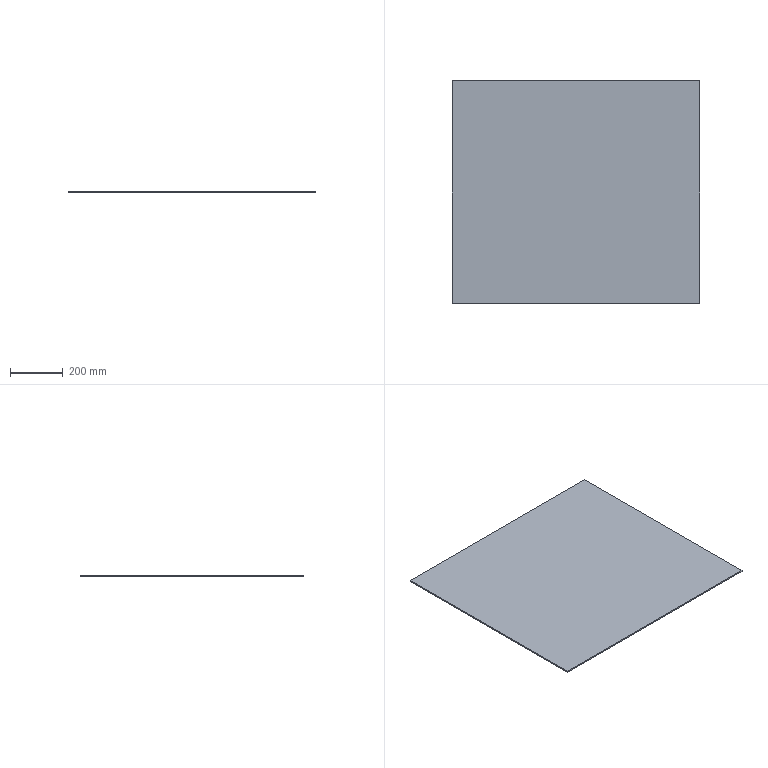Part | SolidWorks | features Extrusion 1, HoleWzd 1 | 1 solid | 6 faces | box 936 x 842 x 5 mm | volume 3940560 mm3 | plane 6
STEP:
#1=CARTESIAN_POINT('',(468.,-421.,0.));
#2=VERTEX_POINT('',#1);
#3=CARTESIAN_POINT('',(468.,421.,0.));
#4=VERTEX_POINT('',#3);
#5=CARTESIAN_POINT('',(468.,421.,0.));
#6=DIRECTION('',(0.,1.,0.));
#7=VECTOR('',#6,1000.);
#8=LINE('',#5,#7);
#9=EDGE_CURVE('',#2,#4,#8,.T.);
#10=ORIENTED_EDGE('',*,*,#9,.T.);
#11=CARTESIAN_POINT('',(468.,421.,5.));
#12=VERTEX_POINT('',#11);
#13=CARTESIAN_POINT('',(468.,421.,5.));
#14=DIRECTION('',(0.,0.,-1.));
#15=VECTOR('',#14,1000.);
#16=LINE('',#13,#15);
#17=EDGE_CURVE('',#12,#4,#16,.T.);
#18=ORIENTED_EDGE('',*,*,#17,.F.);
#19=CARTESIAN_POINT('',(468.,-421.,5.));
#20=VERTEX_POINT('',#19);
#21=CARTESIAN_POINT('',(468.,421.,5.));
#22=DIRECTION('',(0.,1.,0.));
#23=VECTOR('',#22,1000.);
#24=LINE('',#21,#23);
#25=EDGE_CURVE('',#20,#12,#24,.T.);
#26=ORIENTED_EDGE('',*,*,#25,.F.);
#27=CARTESIAN_POINT('',(468.,-421.,5.));
#28=DIRECTION('',(0.,0.,-1.));
#29=VECTOR('',#28,1000.);
#30=LINE('',#27,#29);
#31=EDGE_CURVE('',#20,#2,#30,.T.);
#32=ORIENTED_EDGE('',*,*,#31,.T.);
#33=EDGE_LOOP('',(#10,#18,#26,#32));
#34=FACE_OUTER_BOUND('',#33,.T.);
#35=CARTESIAN_POINT('',(468.,421.,5.));
#36=DIRECTION('',(-1.,0.,0.));
#37=DIRECTION('',(0.,-1.,0.));
#38=AXIS2_PLACEMENT_3D('',#35,#36,#37);
#39=PLANE('',#38);
#40=ADVANCED_FACE('',(#34),#39,.F.);
#41=CARTESIAN_POINT('',(-468.,421.,0.));
#42=VERTEX_POINT('',#41);
#43=CARTESIAN_POINT('',(-468.,421.,0.));
#44=DIRECTION('',(-1.,0.,0.));
#45=VECTOR('',#44,1000.);
#46=LINE('',#43,#45);
#47=EDGE_CURVE('',#4,#42,#46,.T.);
#48=ORIENTED_EDGE('',*,*,#47,.T.);
#49=CARTESIAN_POINT('',(-468.,421.,5.));
#50=VERTEX_POINT('',#49);
#51=CARTESIAN_POINT('',(-468.,421.,5.));
#52=DIRECTION('',(0.,0.,-1.));
#53=VECTOR('',#52,1000.);
#54=LINE('',#51,#53);
#55=EDGE_CURVE('',#50,#42,#54,.T.);
#56=ORIENTED_EDGE('',*,*,#55,.F.);
#57=CARTESIAN_POINT('',(-468.,421.,5.));
#58=DIRECTION('',(-1.,0.,0.));
#59=VECTOR('',#58,1000.);
#60=LINE('',#57,#59);
#61=EDGE_CURVE('',#12,#50,#60,.T.);
#62=ORIENTED_EDGE('',*,*,#61,.F.);
#63=ORIENTED_EDGE('',*,*,#17,.T.);
#64=EDGE_LOOP('',(#48,#56,#62,#63));
#65=FACE_OUTER_BOUND('',#64,.T.);
#66=CARTESIAN_POINT('',(-468.,421.,5.));
#67=DIRECTION('',(0.,-1.,0.));
#68=DIRECTION('',(0.,0.,-1.));
#69=AXIS2_PLACEMENT_3D('',#66,#67,#68);
#70=PLANE('',#69);
#71=ADVANCED_FACE('',(#65),#70,.F.);
#72=CARTESIAN_POINT('',(-468.,-421.,0.));
#73=VERTEX_POINT('',#72);
#74=CARTESIAN_POINT('',(-468.,421.,0.));
#75=DIRECTION('',(0.,-1.,0.));
#76=VECTOR('',#75,1000.);
#77=LINE('',#74,#76);
#78=EDGE_CURVE('',#42,#73,#77,.T.);
#79=ORIENTED_EDGE('',*,*,#78,.T.);
#80=CARTESIAN_POINT('',(-468.,-421.,5.));
#81=VERTEX_POINT('',#80);
#82=CARTESIAN_POINT('',(-468.,-421.,5.));
#83=DIRECTION('',(0.,0.,-1.));
#84=VECTOR('',#83,1000.);
#85=LINE('',#82,#84);
#86=EDGE_CURVE('',#81,#73,#85,.T.);
#87=ORIENTED_EDGE('',*,*,#86,.F.);
#88=CARTESIAN_POINT('',(-468.,421.,5.));
#89=DIRECTION('',(0.,-1.,0.));
#90=VECTOR('',#89,1000.);
#91=LINE('',#88,#90);
#92=EDGE_CURVE('',#50,#81,#91,.T.);
#93=ORIENTED_EDGE('',*,*,#92,.F.);
#94=ORIENTED_EDGE('',*,*,#55,.T.);
#95=EDGE_LOOP('',(#79,#87,#93,#94));
#96=FACE_OUTER_BOUND('',#95,.T.);
#97=CARTESIAN_POINT('',(-468.,421.,5.));
#98=DIRECTION('',(1.,0.,0.));
#99=DIRECTION('',(0.,1.,0.));
#100=AXIS2_PLACEMENT_3D('',#97,#98,#99);
#101=PLANE('',#100);
#102=ADVANCED_FACE('',(#96),#101,.F.);
#103=CARTESIAN_POINT('',(-468.,-421.,0.));
#104=DIRECTION('',(1.,0.,0.));
#105=VECTOR('',#104,1000.);
#106=LINE('',#103,#105);
#107=EDGE_CURVE('',#73,#2,#106,.T.);
#108=ORIENTED_EDGE('',*,*,#107,.T.);
#109=ORIENTED_EDGE('',*,*,#31,.F.);
#110=CARTESIAN_POINT('',(-468.,-421.,5.));
#111=DIRECTION('',(1.,0.,0.));
#112=VECTOR('',#111,1000.);
#113=LINE('',#110,#112);
#114=EDGE_CURVE('',#81,#20,#113,.T.);
#115=ORIENTED_EDGE('',*,*,#114,.F.);
#116=ORIENTED_EDGE('',*,*,#86,.T.);
#117=EDGE_LOOP('',(#108,#109,#115,#116));
#118=FACE_OUTER_BOUND('',#117,.T.);
#119=CARTESIAN_POINT('',(-468.,-421.,5.));
#120=DIRECTION('',(0.,1.,0.));
#121=DIRECTION('',(0.,0.,1.));
#122=AXIS2_PLACEMENT_3D('',#119,#120,#121);
#123=PLANE('',#122);
#124=ADVANCED_FACE('',(#118),#123,.F.);
#125=ORIENTED_EDGE('',*,*,#25,.T.);
#126=ORIENTED_EDGE('',*,*,#61,.T.);
#127=ORIENTED_EDGE('',*,*,#92,.T.);
#128=ORIENTED_EDGE('',*,*,#114,.T.);
#129=EDGE_LOOP('',(#125,#126,#127,#128));
#130=FACE_OUTER_BOUND('',#129,.T.);
#131=CARTESIAN_POINT('',(0.,0.,5.));
#132=DIRECTION('',(0.,0.,1.));
#133=DIRECTION('',(1.,0.,0.));
#134=AXIS2_PLACEMENT_3D('',#131,#132,#133);
#135=PLANE('',#134);
#136=ADVANCED_FACE('',(#130),#135,.T.);
#137=ORIENTED_EDGE('',*,*,#9,.F.);
#138=ORIENTED_EDGE('',*,*,#107,.F.);
#139=ORIENTED_EDGE('',*,*,#78,.F.);
#140=ORIENTED_EDGE('',*,*,#47,.F.);
#141=EDGE_LOOP('',(#137,#138,#139,#140));
#142=FACE_OUTER_BOUND('',#141,.T.);
#143=CARTESIAN_POINT('',(0.,0.,0.));
#144=DIRECTION('',(0.,0.,1.));
#145=DIRECTION('',(1.,0.,0.));
#146=AXIS2_PLACEMENT_3D('',#143,#144,#145);
#147=PLANE('',#146);
#148=ADVANCED_FACE('',(#142),#147,.F.);
#149=CLOSED_SHELL('',(#40,#71,#102,#124,#136,#148));
#150=MANIFOLD_SOLID_BREP('',#149);
#151=CARTESIAN_POINT('',(0.,0.,0.));
#152=DIRECTION('',(0.,0.,1.));
#153=DIRECTION('',(1.,0.,0.));
#154=AXIS2_PLACEMENT_3D('',#151,#152,#153);
#155=(LENGTH_UNIT()NAMED_UNIT(*)SI_UNIT(.MILLI.,.METRE.));
#156=UNCERTAINTY_MEASURE_WITH_UNIT(LENGTH_MEASURE(0.00001),#155,'','');
#157=(NAMED_UNIT(*)PLANE_ANGLE_UNIT()SI_UNIT($,.RADIAN.));
#158=(NAMED_UNIT(*)SI_UNIT($,.STERADIAN.)SOLID_ANGLE_UNIT());
#159=(GEOMETRIC_REPRESENTATION_CONTEXT(3)GLOBAL_UNCERTAINTY_ASSIGNED_CONTEXT((#156))GLOBAL_UNIT_ASSIGNED_CONTEXT((#155,#157,#158))REPRESENTATION_CONTEXT('',''));
#160=ADVANCED_BREP_SHAPE_REPRESENTATION('',(#150,#154),#159);